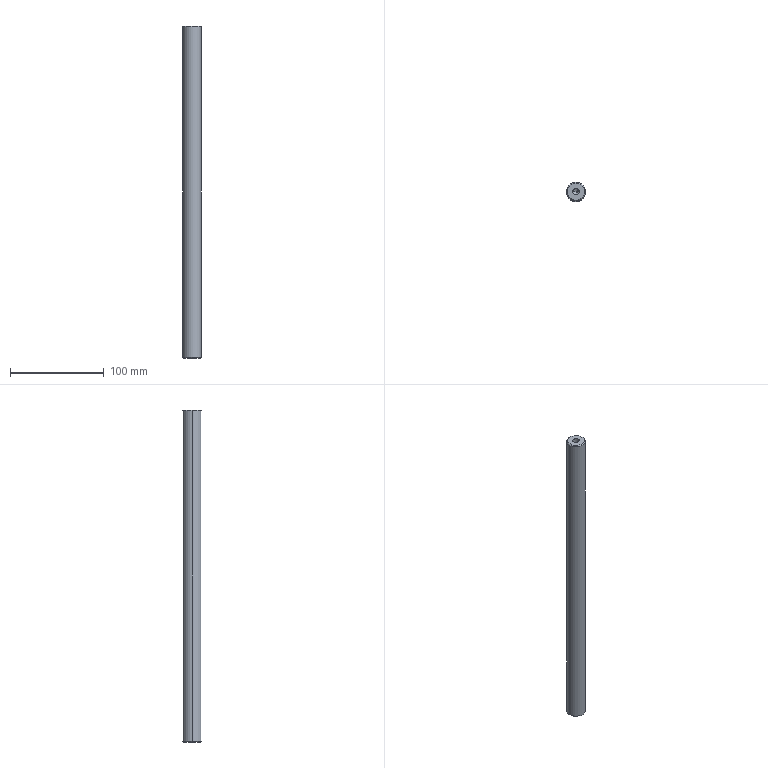Part | SolidWorks | features HoleWzd 2, Chamfer 1, Extrusion 1 | 1 solid | 16 faces | box 20 x 20 x 354 mm | volume 109668 mm3 | cone 8 | cylinder 6 | plane 2 | commonest cylinder face diameters 6.8 x4 20 x2
STEP:
#1=CARTESIAN_POINT('',(9.,0.,177.));
#2=VERTEX_POINT('',#1);
#3=CARTESIAN_POINT('',(-9.,0.,177.));
#4=VERTEX_POINT('',#3);
#5=CARTESIAN_POINT('',(0.,0.,177.));
#6=DIRECTION('',(0.,0.,1.));
#7=DIRECTION('',(1.,0.,0.));
#8=AXIS2_PLACEMENT_3D('',#5,#6,#7);
#9=CIRCLE('',#8,9.);
#10=EDGE_CURVE('',#2,#4,#9,.T.);
#11=ORIENTED_EDGE('',*,*,#10,.F.);
#12=CARTESIAN_POINT('',(10.,0.,176.));
#13=VERTEX_POINT('',#12);
#14=CARTESIAN_POINT('',(9.,0.,177.));
#15=DIRECTION('',(0.7071,0.,-0.7071));
#16=VECTOR('',#15,1000.);
#17=LINE('',#14,#16);
#18=EDGE_CURVE('',#2,#13,#17,.T.);
#19=ORIENTED_EDGE('',*,*,#18,.T.);
#20=CARTESIAN_POINT('',(-10.,0.,176.));
#21=VERTEX_POINT('',#20);
#22=CARTESIAN_POINT('',(0.,0.,176.));
#23=DIRECTION('',(0.,0.,-1.));
#24=DIRECTION('',(1.,0.,0.));
#25=AXIS2_PLACEMENT_3D('',#22,#23,#24);
#26=CIRCLE('',#25,10.);
#27=EDGE_CURVE('',#21,#13,#26,.T.);
#28=ORIENTED_EDGE('',*,*,#27,.F.);
#29=CARTESIAN_POINT('',(-9.,0.,177.));
#30=DIRECTION('',(-0.7071,0.,-0.7071));
#31=VECTOR('',#30,1000.);
#32=LINE('',#29,#31);
#33=EDGE_CURVE('',#4,#21,#32,.T.);
#34=ORIENTED_EDGE('',*,*,#33,.F.);
#35=EDGE_LOOP('',(#11,#19,#28,#34));
#36=FACE_OUTER_BOUND('',#35,.T.);
#37=CARTESIAN_POINT('',(0.,0.,177.));
#38=DIRECTION('',(0.,0.,-1.));
#39=DIRECTION('',(-1.,0.,0.));
#40=AXIS2_PLACEMENT_3D('',#37,#38,#39);
#41=CONICAL_SURFACE('',#40,9.,0.7854);
#42=ADVANCED_FACE('',(#36),#41,.T.);
#43=CARTESIAN_POINT('',(-9.,0.,-177.));
#44=VERTEX_POINT('',#43);
#45=CARTESIAN_POINT('',(9.,0.,-177.));
#46=VERTEX_POINT('',#45);
#47=CARTESIAN_POINT('',(0.,0.,-177.));
#48=DIRECTION('',(0.,0.,-1.));
#49=DIRECTION('',(1.,0.,0.));
#50=AXIS2_PLACEMENT_3D('',#47,#48,#49);
#51=CIRCLE('',#50,9.);
#52=EDGE_CURVE('',#44,#46,#51,.T.);
#53=ORIENTED_EDGE('',*,*,#52,.F.);
#54=CARTESIAN_POINT('',(-10.,0.,-176.));
#55=VERTEX_POINT('',#54);
#56=CARTESIAN_POINT('',(-10.,0.,-176.));
#57=DIRECTION('',(-0.7071,0.,0.7071));
#58=VECTOR('',#57,1000.);
#59=LINE('',#56,#58);
#60=EDGE_CURVE('',#44,#55,#59,.T.);
#61=ORIENTED_EDGE('',*,*,#60,.T.);
#62=CARTESIAN_POINT('',(10.,0.,-176.));
#63=VERTEX_POINT('',#62);
#64=CARTESIAN_POINT('',(0.,0.,-176.));
#65=DIRECTION('',(0.,0.,1.));
#66=DIRECTION('',(1.,0.,0.));
#67=AXIS2_PLACEMENT_3D('',#64,#65,#66);
#68=CIRCLE('',#67,10.);
#69=EDGE_CURVE('',#63,#55,#68,.T.);
#70=ORIENTED_EDGE('',*,*,#69,.F.);
#71=CARTESIAN_POINT('',(10.,0.,-176.));
#72=DIRECTION('',(0.7071,0.,0.7071));
#73=VECTOR('',#72,1000.);
#74=LINE('',#71,#73);
#75=EDGE_CURVE('',#46,#63,#74,.T.);
#76=ORIENTED_EDGE('',*,*,#75,.F.);
#77=EDGE_LOOP('',(#53,#61,#70,#76));
#78=FACE_OUTER_BOUND('',#77,.T.);
#79=CARTESIAN_POINT('',(0.,0.,-176.));
#80=DIRECTION('',(0.,0.,1.));
#81=DIRECTION('',(1.,0.,0.));
#82=AXIS2_PLACEMENT_3D('',#79,#80,#81);
#83=CONICAL_SURFACE('',#82,10.,0.7854);
#84=ADVANCED_FACE('',(#78),#83,.T.);
#85=CARTESIAN_POINT('',(-3.4,0.,157.25));
#86=VERTEX_POINT('',#85);
#87=CARTESIAN_POINT('',(3.4,0.,157.25));
#88=VERTEX_POINT('',#87);
#89=CARTESIAN_POINT('',(0.,0.,157.25));
#90=DIRECTION('',(0.,0.,1.));
#91=DIRECTION('',(1.,0.,0.));
#92=AXIS2_PLACEMENT_3D('',#89,#90,#91);
#93=CIRCLE('',#92,3.4);
#94=EDGE_CURVE('',#86,#88,#93,.T.);
#95=ORIENTED_EDGE('',*,*,#94,.F.);
#96=CARTESIAN_POINT('',(-3.4,0.,177.));
#97=VERTEX_POINT('',#96);
#98=CARTESIAN_POINT('',(-3.4,0.,177.));
#99=DIRECTION('',(0.,0.,1.));
#100=VECTOR('',#99,1000.);
#101=LINE('',#98,#100);
#102=EDGE_CURVE('',#86,#97,#101,.T.);
#103=ORIENTED_EDGE('',*,*,#102,.T.);
#104=CARTESIAN_POINT('',(3.4,0.,177.));
#105=VERTEX_POINT('',#104);
#106=CARTESIAN_POINT('',(0.,0.,177.));
#107=DIRECTION('',(0.,0.,1.));
#108=DIRECTION('',(1.,0.,0.));
#109=AXIS2_PLACEMENT_3D('',#106,#107,#108);
#110=CIRCLE('',#109,3.4);
#111=EDGE_CURVE('',#97,#105,#110,.T.);
#112=ORIENTED_EDGE('',*,*,#111,.T.);
#113=CARTESIAN_POINT('',(3.4,0.,177.));
#114=DIRECTION('',(0.,0.,1.));
#115=VECTOR('',#114,1000.);
#116=LINE('',#113,#115);
#117=EDGE_CURVE('',#88,#105,#116,.T.);
#118=ORIENTED_EDGE('',*,*,#117,.F.);
#119=EDGE_LOOP('',(#95,#103,#112,#118));
#120=FACE_OUTER_BOUND('',#119,.T.);
#121=CARTESIAN_POINT('',(0.,0.,177.));
#122=DIRECTION('',(0.,0.,1.));
#123=DIRECTION('',(1.,0.,0.));
#124=AXIS2_PLACEMENT_3D('',#121,#122,#123);
#125=CYLINDRICAL_SURFACE('',#124,3.4);
#126=ADVANCED_FACE('',(#120),#125,.F.);
#127=CARTESIAN_POINT('',(0.,0.,155.207));
#128=VERTEX_POINT('',#127);
#129=CARTESIAN_POINT('',(3.4,0.,157.25));
#130=DIRECTION('',(0.8572,0.,0.515));
#131=VECTOR('',#130,1000.);
#132=LINE('',#129,#131);
#133=EDGE_CURVE('',#128,#88,#132,.T.);
#134=ORIENTED_EDGE('',*,*,#133,.F.);
#135=CARTESIAN_POINT('',(-3.4,0.,157.25));
#136=DIRECTION('',(-0.8572,0.,0.515));
#137=VECTOR('',#136,1000.);
#138=LINE('',#135,#137);
#139=EDGE_CURVE('',#128,#86,#138,.T.);
#140=ORIENTED_EDGE('',*,*,#139,.T.);
#141=ORIENTED_EDGE('',*,*,#94,.T.);
#142=EDGE_LOOP('',(#134,#140,#141));
#143=FACE_OUTER_BOUND('',#142,.T.);
#144=CARTESIAN_POINT('',(0.,0.,157.25));
#145=DIRECTION('',(0.,0.,1.));
#146=DIRECTION('',(1.,0.,0.));
#147=AXIS2_PLACEMENT_3D('',#144,#145,#146);
#148=CONICAL_SURFACE('',#147,3.4,1.03);
#149=ADVANCED_FACE('',(#143),#148,.F.);
#150=CARTESIAN_POINT('',(3.4,0.,-157.25));
#151=VERTEX_POINT('',#150);
#152=CARTESIAN_POINT('',(-3.4,0.,-157.25));
#153=VERTEX_POINT('',#152);
#154=CARTESIAN_POINT('',(0.,0.,-157.25));
#155=DIRECTION('',(0.,0.,-1.));
#156=DIRECTION('',(-1.,0.,0.));
#157=AXIS2_PLACEMENT_3D('',#154,#155,#156);
#158=CIRCLE('',#157,3.4);
#159=EDGE_CURVE('',#151,#153,#158,.T.);
#160=ORIENTED_EDGE('',*,*,#159,.F.);
#161=CARTESIAN_POINT('',(3.4,0.,-177.));
#162=VERTEX_POINT('',#161);
#163=CARTESIAN_POINT('',(3.4,0.,-177.));
#164=DIRECTION('',(0.,0.,-1.));
#165=VECTOR('',#164,1000.);
#166=LINE('',#163,#165);
#167=EDGE_CURVE('',#151,#162,#166,.T.);
#168=ORIENTED_EDGE('',*,*,#167,.T.);
#169=CARTESIAN_POINT('',(-3.4,0.,-177.));
#170=VERTEX_POINT('',#169);
#171=CARTESIAN_POINT('',(0.,0.,-177.));
#172=DIRECTION('',(0.,0.,-1.));
#173=DIRECTION('',(-1.,0.,0.));
#174=AXIS2_PLACEMENT_3D('',#171,#172,#173);
#175=CIRCLE('',#174,3.4);
#176=EDGE_CURVE('',#162,#170,#175,.T.);
#177=ORIENTED_EDGE('',*,*,#176,.T.);
#178=CARTESIAN_POINT('',(-3.4,0.,-177.));
#179=DIRECTION('',(0.,0.,-1.));
#180=VECTOR('',#179,1000.);
#181=LINE('',#178,#180);
#182=EDGE_CURVE('',#153,#170,#181,.T.);
#183=ORIENTED_EDGE('',*,*,#182,.F.);
#184=EDGE_LOOP('',(#160,#168,#177,#183));
#185=FACE_OUTER_BOUND('',#184,.T.);
#186=CARTESIAN_POINT('',(0.,0.,-177.));
#187=DIRECTION('',(0.,0.,-1.));
#188=DIRECTION('',(-1.,0.,0.));
#189=AXIS2_PLACEMENT_3D('',#186,#187,#188);
#190=CYLINDRICAL_SURFACE('',#189,3.4);
#191=ADVANCED_FACE('',(#185),#190,.F.);
#192=CARTESIAN_POINT('',(0.,0.,-155.207));
#193=VERTEX_POINT('',#192);
#194=CARTESIAN_POINT('',(-3.4,0.,-157.25));
#195=DIRECTION('',(-0.8572,0.,-0.515));
#196=VECTOR('',#195,1000.);
#197=LINE('',#194,#196);
#198=EDGE_CURVE('',#193,#153,#197,.T.);
#199=ORIENTED_EDGE('',*,*,#198,.F.);
#200=CARTESIAN_POINT('',(3.4,0.,-157.25));
#201=DIRECTION('',(0.8572,0.,-0.515));
#202=VECTOR('',#201,1000.);
#203=LINE('',#200,#202);
#204=EDGE_CURVE('',#193,#151,#203,.T.);
#205=ORIENTED_EDGE('',*,*,#204,.T.);
#206=ORIENTED_EDGE('',*,*,#159,.T.);
#207=EDGE_LOOP('',(#199,#205,#206));
#208=FACE_OUTER_BOUND('',#207,.T.);
#209=CARTESIAN_POINT('',(0.,0.,-157.25));
#210=DIRECTION('',(0.,0.,-1.));
#211=DIRECTION('',(-1.,0.,0.));
#212=AXIS2_PLACEMENT_3D('',#209,#210,#211);
#213=CONICAL_SURFACE('',#212,3.4,1.03);
#214=ADVANCED_FACE('',(#208),#213,.F.);
#215=ORIENTED_EDGE('',*,*,#27,.T.);
#216=CARTESIAN_POINT('',(10.,0.,177.));
#217=DIRECTION('',(0.,0.,-1.));
#218=VECTOR('',#217,1000.);
#219=LINE('',#216,#218);
#220=EDGE_CURVE('',#13,#63,#219,.T.);
#221=ORIENTED_EDGE('',*,*,#220,.T.);
#222=ORIENTED_EDGE('',*,*,#69,.T.);
#223=CARTESIAN_POINT('',(-10.,0.,177.));
#224=DIRECTION('',(0.,0.,-1.));
#225=VECTOR('',#224,1000.);
#226=LINE('',#223,#225);
#227=EDGE_CURVE('',#21,#55,#226,.T.);
#228=ORIENTED_EDGE('',*,*,#227,.F.);
#229=EDGE_LOOP('',(#215,#221,#222,#228));
#230=FACE_OUTER_BOUND('',#229,.T.);
#231=CARTESIAN_POINT('',(0.,0.,177.));
#232=DIRECTION('',(0.,0.,-1.));
#233=DIRECTION('',(-1.,0.,0.));
#234=AXIS2_PLACEMENT_3D('',#231,#232,#233);
#235=CYLINDRICAL_SURFACE('',#234,10.);
#236=ADVANCED_FACE('',(#230),#235,.T.);
#237=ORIENTED_EDGE('',*,*,#220,.F.);
#238=CARTESIAN_POINT('',(0.,0.,176.));
#239=DIRECTION('',(0.,0.,-1.));
#240=DIRECTION('',(1.,0.,0.));
#241=AXIS2_PLACEMENT_3D('',#238,#239,#240);
#242=CIRCLE('',#241,10.);
#243=EDGE_CURVE('',#13,#21,#242,.T.);
#244=ORIENTED_EDGE('',*,*,#243,.T.);
#245=ORIENTED_EDGE('',*,*,#227,.T.);
#246=CARTESIAN_POINT('',(0.,0.,-176.));
#247=DIRECTION('',(0.,0.,1.));
#248=DIRECTION('',(1.,0.,0.));
#249=AXIS2_PLACEMENT_3D('',#246,#247,#248);
#250=CIRCLE('',#249,10.);
#251=EDGE_CURVE('',#55,#63,#250,.T.);
#252=ORIENTED_EDGE('',*,*,#251,.T.);
#253=EDGE_LOOP('',(#237,#244,#245,#252));
#254=FACE_OUTER_BOUND('',#253,.T.);
#255=CARTESIAN_POINT('',(0.,0.,177.));
#256=DIRECTION('',(0.,0.,-1.));
#257=DIRECTION('',(-1.,0.,0.));
#258=AXIS2_PLACEMENT_3D('',#255,#256,#257);
#259=CYLINDRICAL_SURFACE('',#258,10.);
#260=ADVANCED_FACE('',(#254),#259,.T.);
#261=CARTESIAN_POINT('',(0.,0.,177.));
#262=DIRECTION('',(0.,0.,1.));
#263=DIRECTION('',(1.,0.,0.));
#264=AXIS2_PLACEMENT_3D('',#261,#262,#263);
#265=CIRCLE('',#264,9.);
#266=EDGE_CURVE('',#4,#2,#265,.T.);
#267=ORIENTED_EDGE('',*,*,#266,.T.);
#268=ORIENTED_EDGE('',*,*,#10,.T.);
#269=EDGE_LOOP('',(#267,#268));
#270=FACE_OUTER_BOUND('',#269,.T.);
#271=CARTESIAN_POINT('',(0.,0.,177.));
#272=DIRECTION('',(0.,0.,1.));
#273=DIRECTION('',(1.,0.,0.));
#274=AXIS2_PLACEMENT_3D('',#271,#272,#273);
#275=CIRCLE('',#274,3.4);
#276=EDGE_CURVE('',#105,#97,#275,.T.);
#277=ORIENTED_EDGE('',*,*,#276,.F.);
#278=ORIENTED_EDGE('',*,*,#111,.F.);
#279=EDGE_LOOP('',(#277,#278));
#280=FACE_BOUND('',#279,.T.);
#281=CARTESIAN_POINT('',(0.,0.,177.));
#282=DIRECTION('',(0.,0.,1.));
#283=DIRECTION('',(1.,0.,0.));
#284=AXIS2_PLACEMENT_3D('',#281,#282,#283);
#285=PLANE('',#284);
#286=ADVANCED_FACE('',(#270,#280),#285,.T.);
#287=CARTESIAN_POINT('',(0.,0.,-177.));
#288=DIRECTION('',(0.,0.,-1.));
#289=DIRECTION('',(1.,0.,0.));
#290=AXIS2_PLACEMENT_3D('',#287,#288,#289);
#291=CIRCLE('',#290,9.);
#292=EDGE_CURVE('',#46,#44,#291,.T.);
#293=ORIENTED_EDGE('',*,*,#292,.T.);
#294=ORIENTED_EDGE('',*,*,#52,.T.);
#295=EDGE_LOOP('',(#293,#294));
#296=FACE_OUTER_BOUND('',#295,.T.);
#297=CARTESIAN_POINT('',(0.,0.,-177.));
#298=DIRECTION('',(0.,0.,-1.));
#299=DIRECTION('',(-1.,0.,0.));
#300=AXIS2_PLACEMENT_3D('',#297,#298,#299);
#301=CIRCLE('',#300,3.4);
#302=EDGE_CURVE('',#170,#162,#301,.T.);
#303=ORIENTED_EDGE('',*,*,#302,.F.);
#304=ORIENTED_EDGE('',*,*,#176,.F.);
#305=EDGE_LOOP('',(#303,#304));
#306=FACE_BOUND('',#305,.T.);
#307=CARTESIAN_POINT('',(0.,0.,-177.));
#308=DIRECTION('',(0.,0.,1.));
#309=DIRECTION('',(1.,0.,0.));
#310=AXIS2_PLACEMENT_3D('',#307,#308,#309);
#311=PLANE('',#310);
#312=ADVANCED_FACE('',(#296,#306),#311,.F.);
#313=ORIENTED_EDGE('',*,*,#204,.F.);
#314=ORIENTED_EDGE('',*,*,#198,.T.);
#315=CARTESIAN_POINT('',(0.,0.,-157.25));
#316=DIRECTION('',(0.,0.,-1.));
#317=DIRECTION('',(-1.,0.,0.));
#318=AXIS2_PLACEMENT_3D('',#315,#316,#317);
#319=CIRCLE('',#318,3.4);
#320=EDGE_CURVE('',#153,#151,#319,.T.);
#321=ORIENTED_EDGE('',*,*,#320,.T.);
#322=EDGE_LOOP('',(#313,#314,#321));
#323=FACE_OUTER_BOUND('',#322,.T.);
#324=CARTESIAN_POINT('',(0.,0.,-157.25));
#325=DIRECTION('',(0.,0.,-1.));
#326=DIRECTION('',(-1.,0.,0.));
#327=AXIS2_PLACEMENT_3D('',#324,#325,#326);
#328=CONICAL_SURFACE('',#327,3.4,1.03);
#329=ADVANCED_FACE('',(#323),#328,.F.);
#330=ORIENTED_EDGE('',*,*,#167,.F.);
#331=ORIENTED_EDGE('',*,*,#320,.F.);
#332=ORIENTED_EDGE('',*,*,#182,.T.);
#333=ORIENTED_EDGE('',*,*,#302,.T.);
#334=EDGE_LOOP('',(#330,#331,#332,#333));
#335=FACE_OUTER_BOUND('',#334,.T.);
#336=CARTESIAN_POINT('',(0.,0.,-177.));
#337=DIRECTION('',(0.,0.,-1.));
#338=DIRECTION('',(-1.,0.,0.));
#339=AXIS2_PLACEMENT_3D('',#336,#337,#338);
#340=CYLINDRICAL_SURFACE('',#339,3.4);
#341=ADVANCED_FACE('',(#335),#340,.F.);
#342=ORIENTED_EDGE('',*,*,#139,.F.);
#343=ORIENTED_EDGE('',*,*,#133,.T.);
#344=CARTESIAN_POINT('',(0.,0.,157.25));
#345=DIRECTION('',(0.,0.,1.));
#346=DIRECTION('',(1.,0.,0.));
#347=AXIS2_PLACEMENT_3D('',#344,#345,#346);
#348=CIRCLE('',#347,3.4);
#349=EDGE_CURVE('',#88,#86,#348,.T.);
#350=ORIENTED_EDGE('',*,*,#349,.T.);
#351=EDGE_LOOP('',(#342,#343,#350));
#352=FACE_OUTER_BOUND('',#351,.T.);
#353=CARTESIAN_POINT('',(0.,0.,157.25));
#354=DIRECTION('',(0.,0.,1.));
#355=DIRECTION('',(1.,0.,0.));
#356=AXIS2_PLACEMENT_3D('',#353,#354,#355);
#357=CONICAL_SURFACE('',#356,3.4,1.03);
#358=ADVANCED_FACE('',(#352),#357,.F.);
#359=ORIENTED_EDGE('',*,*,#102,.F.);
#360=ORIENTED_EDGE('',*,*,#349,.F.);
#361=ORIENTED_EDGE('',*,*,#117,.T.);
#362=ORIENTED_EDGE('',*,*,#276,.T.);
#363=EDGE_LOOP('',(#359,#360,#361,#362));
#364=FACE_OUTER_BOUND('',#363,.T.);
#365=CARTESIAN_POINT('',(0.,0.,177.));
#366=DIRECTION('',(0.,0.,1.));
#367=DIRECTION('',(1.,0.,0.));
#368=AXIS2_PLACEMENT_3D('',#365,#366,#367);
#369=CYLINDRICAL_SURFACE('',#368,3.4);
#370=ADVANCED_FACE('',(#364),#369,.F.);
#371=ORIENTED_EDGE('',*,*,#60,.F.);
#372=ORIENTED_EDGE('',*,*,#292,.F.);
#373=ORIENTED_EDGE('',*,*,#75,.T.);
#374=ORIENTED_EDGE('',*,*,#251,.F.);
#375=EDGE_LOOP('',(#371,#372,#373,#374));
#376=FACE_OUTER_BOUND('',#375,.T.);
#377=CARTESIAN_POINT('',(0.,0.,-176.));
#378=DIRECTION('',(0.,0.,1.));
#379=DIRECTION('',(1.,0.,0.));
#380=AXIS2_PLACEMENT_3D('',#377,#378,#379);
#381=CONICAL_SURFACE('',#380,10.,0.7854);
#382=ADVANCED_FACE('',(#376),#381,.T.);
#383=ORIENTED_EDGE('',*,*,#18,.F.);
#384=ORIENTED_EDGE('',*,*,#266,.F.);
#385=ORIENTED_EDGE('',*,*,#33,.T.);
#386=ORIENTED_EDGE('',*,*,#243,.F.);
#387=EDGE_LOOP('',(#383,#384,#385,#386));
#388=FACE_OUTER_BOUND('',#387,.T.);
#389=CARTESIAN_POINT('',(0.,0.,177.));
#390=DIRECTION('',(0.,0.,-1.));
#391=DIRECTION('',(-1.,0.,0.));
#392=AXIS2_PLACEMENT_3D('',#389,#390,#391);
#393=CONICAL_SURFACE('',#392,9.,0.7854);
#394=ADVANCED_FACE('',(#388),#393,.T.);
#395=CLOSED_SHELL('',(#42,#84,#126,#149,#191,#214,#236,#260,#286,#312,#329,#341,#358,#370,#382,#394));
#396=MANIFOLD_SOLID_BREP('',#395);
#397=CARTESIAN_POINT('',(0.,0.,0.));
#398=DIRECTION('',(0.,0.,1.));
#399=DIRECTION('',(1.,0.,0.));
#400=AXIS2_PLACEMENT_3D('',#397,#398,#399);
#401=(LENGTH_UNIT()NAMED_UNIT(*)SI_UNIT(.MILLI.,.METRE.));
#402=UNCERTAINTY_MEASURE_WITH_UNIT(LENGTH_MEASURE(0.00001),#401,'','');
#403=(NAMED_UNIT(*)PLANE_ANGLE_UNIT()SI_UNIT($,.RADIAN.));
#404=(NAMED_UNIT(*)SI_UNIT($,.STERADIAN.)SOLID_ANGLE_UNIT());
#405=(GEOMETRIC_REPRESENTATION_CONTEXT(3)GLOBAL_UNCERTAINTY_ASSIGNED_CONTEXT((#402))GLOBAL_UNIT_ASSIGNED_CONTEXT((#401,#403,#404))REPRESENTATION_CONTEXT('',''));
#406=ADVANCED_BREP_SHAPE_REPRESENTATION('',(#396,#400),#405);